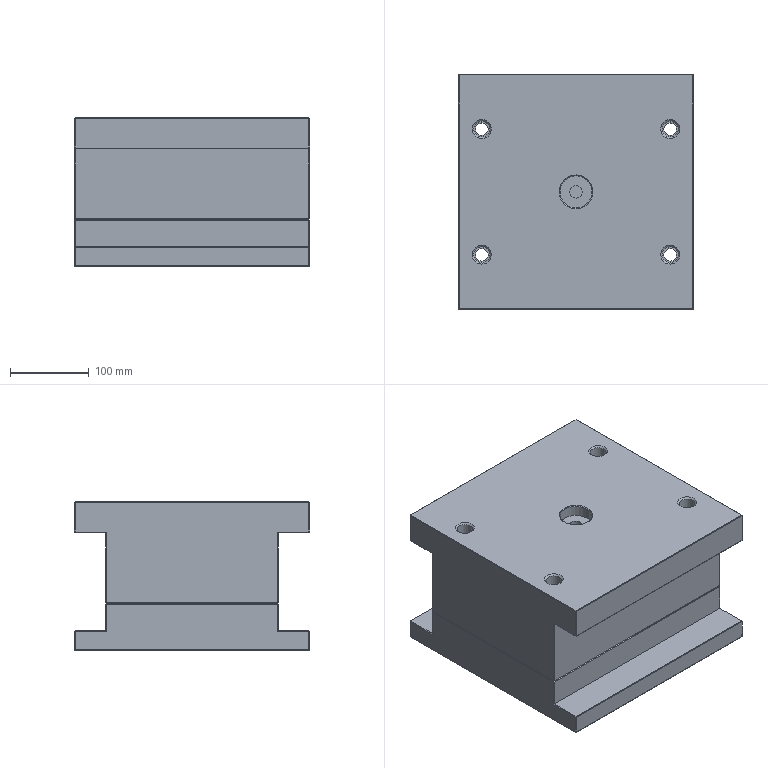NC program | NX | posted with a generic post | part box 300 x 300 x 190 mm
Lines 33368 to 33426 of 34829:
(FLOOR_WALL_1_COPY_1 , TOOL : D25R0.8)
N66728 T15 M6
N66730 G54
N66732 G17 G0 G90 X163.665 Y-150.247 S4000 M3
N66734 G43 Z30. H15
N66736 Z-88.5
N66738 G94 G1 Z-90. F800.
N66740 G3 X161.5 Y-148.997 R2.5
N66742 G1 X-161.5
N66744 Y-140.588
N66746 X161.5
N66748 Y-132.179
N66750 X-161.5
N66752 Y-123.77
N66754 X161.5
N66756 G2 X163.665 Y-125.02 R2.5
N66758 G1 Z-88.5
N66760 G0 Z30.
N66762 X164.1 Y-114.722
N66764 Z-88.5
N66766 G1 Z-90.
N66768 X163.915 Y-114.672
N66770 G3 X161.5 Y-115.319 R2.5
N66772 G1 X154.219 Y-122.6
N66774 X-154.219
N66776 X-161.5 Y-115.319
N66778 G3 X-163.915 Y-114.672 R2.5
N66780 G1 X-164.1 Y-114.722
N66782 Z-88.5
N66784 G0 Z30.
N66786 X-163.665 Y150.247
N66788 Z-88.5
N66790 G1 Z-90.
N66792 G3 X-161.5 Y148.997 R2.5
N66794 G1 X161.5
N66796 Y140.588
N66798 X-161.5
N66800 Y132.179
N66802 X161.5
N66804 Y123.77
N66806 X-161.5
N66808 G2 X-163.665 Y125.02 R2.5
N66810 G1 Z-88.5
N66812 G0 Z30.
N66814 X-164.1 Y114.722
N66816 Z-88.5
N66818 G1 Z-90.
N66820 X-163.915 Y114.672
N66822 G3 X-161.5 Y115.319 R2.5
N66824 G1 X-154.219 Y122.6
N66826 X154.219
N66828 X161.5 Y115.319
N66830 G3 X163.915 Y114.672 R2.5
N66832 G1 X164.1 Y114.722
N66834 Z-88.5
N66836 G0 Z30.
N66838 M5